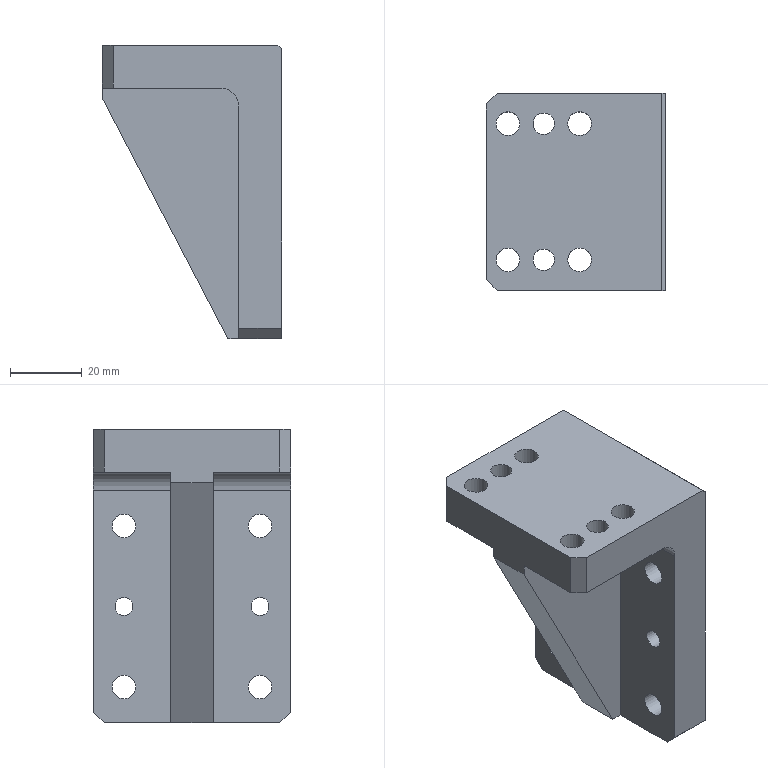CAM job | NX | 3+2 milling, drilling | part box 50 x 55 x 82 mm | stock box 55 x 60 x 87 mm
Tools:
number,name,description,diameter,corner_radius,flute_length,length,flutes
9,D10,平底铣刀-粗,10.0,0.0,35.0,75.0,2
7,D6-J,平底铣刀-精,6.0,0.0,25.0,75.0,2
10,D10-J,平底铣刀-精,10.0,0.0,35.0,75.0,2
17,D6R0.5,圆鼻刀-粗,6.0,0.5,50.0,75.0,2
1,D80R0.8飞刀,圆鼻刀-粗,80.0,0.8,50.0,75.0,2
1,D80R0.8飞刀-J,圆鼻刀-精,80.0,0.8,50.0,75.0,2
2,D6倒角刀,倒角刀,6.0,0.0,3.0,25.0,2
19,D5铰刀,Drilling Tool,5.0,0.0,75.0,100.0,6
18,DRILL6.6,Drilling Tool,6.6,0.0,35.0,50.0,2
17,ZT4.9,Drilling Tool,4.9,0.0,35.0,50.0,2
Operations:
program,operation,operation_type,tool,method,geometry_group,spindle_rpm,surface_speed,feed_per_tooth,feed_cut,feed_plunge,cut_length_mm,path_length_mm,cut_time_min,machine_time_min
B,FLOORWALLFACEMILLONECUTROUGH_COPY,VolumeBased25DMillingOperation,D80R0.8飞刀,LAYERROUGH-DEPTHK-STEPG,W-B,2800.0,703.696,0.5357,3000.0,100.0,1711.746,3759.967,0.5706,0.7754
B,FLOORWALLFACEMILLONECUTFINISH_COPY,VolumeBased25DMillingOperation,D80R0.8飞刀-J,SIDEFINISH-DEPTHK-STEPG,W-B,4000.0,1005.28,0.125,1000.0,100.0,189.998,285.998,0.19,0.1996
B,CAVITYROUGH-MED_COPY,CavityMilling,D10,LAYERROUGH-DEPTHK-STEPG,W-B,8000.0,251.32,0.25,4000.0,100.0,51360.027,54446.807,12.84,13.293
B,PLANARDEBURR6X45L_COPY,SurfaceContour,D6倒角刀,WALLCLIMB_CHAMFER-DEPTH0-STEPG,W-B,6500.0,122.519,0.1154,1500.0,100.0,381.524,1587.457,0.2543,0.3749
B,ZLEVELFINISHZIGZAGCLIMB_COPY,ZLevelMilling,D6R0.5,ZLEVELWALLCLIMB-DEPTHK-STEPG,W-B,7000.0,131.947,0.2857,4000.0,100.0,1436.438,1561.706,0.3591,0.3716
B,ZLEVELFINISHZIGZAGCLIMB_COPY_COPY,ZLevelMilling,D6R0.5,ZLEVELWALLCLIMB-DEPTHK-STEPG,W-B,7000.0,131.947,0.2857,4000.0,100.0,10969.644,11033.69,2.742,2.749
B,FLOORWALLFINISHBOTTOM-MED_COPY,VolumeBased25DMillingOperation,D6-J,FINISHSTEPDEPTHOFF,W-B,7000.0,175.0,0.0536,1500.0,100.0,1028.407,1284.561,0.6856,0.7112
B,ZLEVELSMOOTHCORNERD6REF12_COPY,ZLevelMilling,D6-J,LAYERFINISH-DEPTHK-STEPG,W-B,8000.0,150.796,0.125,2000.0,100.0,3295.978,3590.017,1.648,1.677
B,ZLEVELFINISH-MED_COPY,ZLevelMilling,D6-J,SIDEFINISH-DEPTHK-STEPG,W-B,8000.0,150.792,0.0625,1000.0,100.0,890.12,1616.806,0.8901,0.9628
B,ZLEVELFINISHZIGZAGCLIMB_COPY_1,ZLevelMilling,D6-J,ZLEVELWALLCLIMB-DEPTHK-STEPG,W-B,7000.0,131.947,0.25,3500.0,100.0,19080.145,19328.011,5.452,5.476
A,TOPFACE,FaceMilling,D80R0.8飞刀,SIDEFINISH-DEPTHK-STEPG,W-A,4500.0,1385.0,0.1667,1500.0,100.0,176.0,272.0,0.1173,0.1269
A,SPOT-DEPTH0.8,Operation,D6倒角刀,NONE,W-A,8000.0,150.796,0.0312,500.0,90.0,10.8,254.702,0.0216,0.046
A,THRUHOLE-PREDRILL6.0,Operation,ZT4.9,NONE,W-A,2500.0,38.484,0.05,250.0,90.0,34.829,208.671,0.1393,0.1567
A,THRUHOLE-6-8,Operation,DRILL6.6,NONE,W-A,2500.0,51.836,0.03,150.0,90.0,67.621,359.279,0.4508,0.48
A,PROFILEROUGH_2,VolumeBased25DMillingOperation,D10,METHOD,W-A,6000.0,188.496,0.5,6000.0,80.0,19665.985,19814.485,3.278,3.292
A,BODYONLY,SurfaceContour,D6倒角刀,METHOD,W-A,8000.0,150.796,0.1875,3000.0,100.0,227.378,321.509,0.0758,0.0852
A,MILLCHAMFER_1,PlanarMilling,D6倒角刀,METHOD,W-A,8000.0,150.796,0.0312,500.0,100.0,36.963,278.532,0.0739,0.0981
A,MILLCHAMFER_2,PlanarMilling,D6倒角刀,METHOD,W-A,8000.0,150.796,0.05,800.0,100.0,92.54,617.64,0.1157,0.1682
A,FLOORWALLCHAMFER_COPY,VolumeBased25DMillingOperation,D6倒角刀,WALLCLIMB_CHAMFER-DEPTH0-STEPG,W-A,6500.0,122.519,0.1154,1500.0,100.0,63.801,164.201,0.0425,0.0526
A,REAM,Operation,D5铰刀,METHOD,W-A,500.0,7.854,0.0167,50.0,0.0,28.0,195.013,0.56,0.5767
A,PROFILESEMI_2,VolumeBased25DMillingOperation,D10-J,METHOD,W-A,9000.0,169.646,0.0667,1200.0,100.0,1534.297,2339.355,1.279,1.359